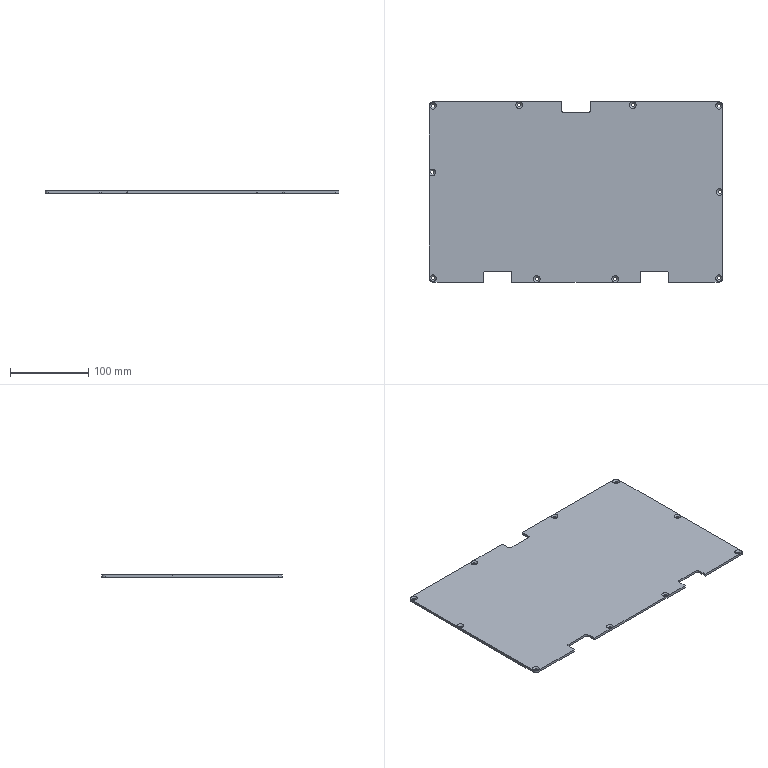Part | SolidWorks | features BaseBody 1, HoleWzd 1, MoveFace 1 | 1 solid | 68 faces | box 375 x 230 x 3 mm | volume 253484 mm3 | cylinder 30 | cone 20 | plane 18 | commonest cylinder face diameters 4.5 x20 4 x6 10 x4